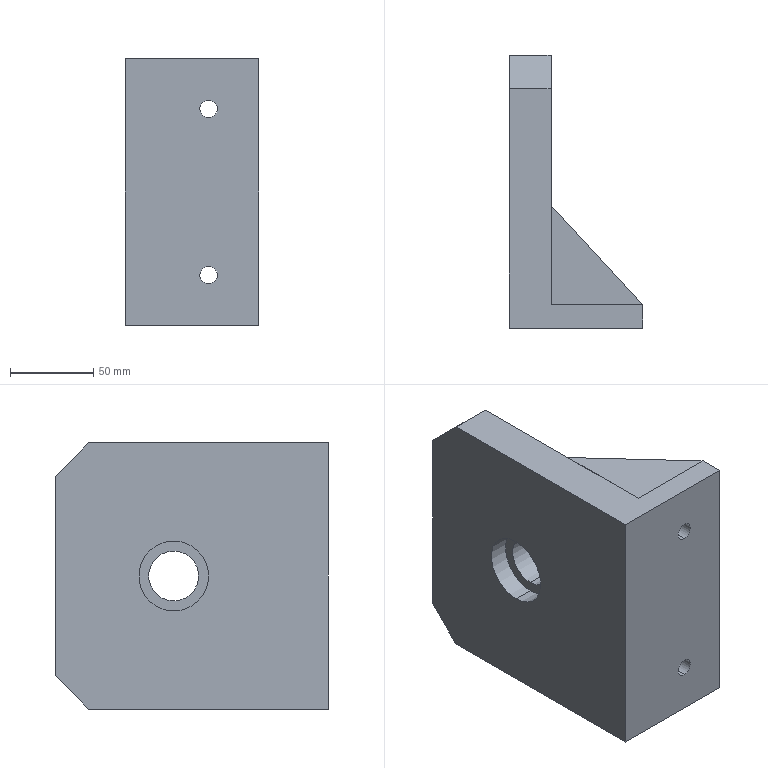Part | SolidWorks | features ICE 5, Chamfer 1, Extrusion 1, HoleWzd 1 | 3 solids | 29 faces | box 80 x 164 x 160 mm | volume 773961 mm3 | plane 21 | cylinder 8 | commonest cylinder face diameters 10.5 x4 30 x2 42 x2
STEP:
#1=CARTESIAN_POINT('',(-15.,74.,80.));
#2=VERTEX_POINT('',#1);
#3=CARTESIAN_POINT('',(-15.,14.,80.));
#4=VERTEX_POINT('',#3);
#5=CARTESIAN_POINT('',(-15.,74.,80.));
#6=DIRECTION('',(0.,-1.,0.));
#7=VECTOR('',#6,1000.);
#8=LINE('',#5,#7);
#9=EDGE_CURVE('',#2,#4,#8,.T.);
#10=ORIENTED_EDGE('',*,*,#9,.F.);
#11=CARTESIAN_POINT('',(-15.,74.,70.));
#12=VERTEX_POINT('',#11);
#13=CARTESIAN_POINT('',(-15.,74.,70.));
#14=DIRECTION('',(0.,0.,1.));
#15=VECTOR('',#14,1000.);
#16=LINE('',#13,#15);
#17=EDGE_CURVE('',#12,#2,#16,.T.);
#18=ORIENTED_EDGE('',*,*,#17,.F.);
#19=CARTESIAN_POINT('',(-15.,14.,70.));
#20=VERTEX_POINT('',#19);
#21=CARTESIAN_POINT('',(-15.,74.,70.));
#22=DIRECTION('',(0.,-1.,0.));
#23=VECTOR('',#22,1000.);
#24=LINE('',#21,#23);
#25=EDGE_CURVE('',#12,#20,#24,.T.);
#26=ORIENTED_EDGE('',*,*,#25,.T.);
#27=CARTESIAN_POINT('',(-15.,14.,70.));
#28=DIRECTION('',(0.,0.,1.));
#29=VECTOR('',#28,1000.);
#30=LINE('',#27,#29);
#31=EDGE_CURVE('',#20,#4,#30,.T.);
#32=ORIENTED_EDGE('',*,*,#31,.T.);
#33=EDGE_LOOP('',(#10,#18,#26,#32));
#34=FACE_OUTER_BOUND('',#33,.T.);
#35=CARTESIAN_POINT('',(-15.,74.,70.));
#36=DIRECTION('',(-1.,0.,0.));
#37=DIRECTION('',(0.,-1.,0.));
#38=AXIS2_PLACEMENT_3D('',#35,#36,#37);
#39=PLANE('',#38);
#40=ADVANCED_FACE('',(#34),#39,.T.);
#41=CARTESIAN_POINT('',(40.,14.,80.));
#42=VERTEX_POINT('',#41);
#43=CARTESIAN_POINT('',(-15.,74.,80.));
#44=DIRECTION('',(-0.6757,0.7372,0.));
#45=VECTOR('',#44,1000.);
#46=LINE('',#43,#45);
#47=EDGE_CURVE('',#42,#2,#46,.T.);
#48=ORIENTED_EDGE('',*,*,#47,.F.);
#49=CARTESIAN_POINT('',(40.,14.,70.));
#50=VERTEX_POINT('',#49);
#51=CARTESIAN_POINT('',(40.,14.,70.));
#52=DIRECTION('',(0.,0.,1.));
#53=VECTOR('',#52,1000.);
#54=LINE('',#51,#53);
#55=EDGE_CURVE('',#50,#42,#54,.T.);
#56=ORIENTED_EDGE('',*,*,#55,.F.);
#57=CARTESIAN_POINT('',(-15.,74.,70.));
#58=DIRECTION('',(-0.6757,0.7372,0.));
#59=VECTOR('',#58,1000.);
#60=LINE('',#57,#59);
#61=EDGE_CURVE('',#50,#12,#60,.T.);
#62=ORIENTED_EDGE('',*,*,#61,.T.);
#63=ORIENTED_EDGE('',*,*,#17,.T.);
#64=EDGE_LOOP('',(#48,#56,#62,#63));
#65=FACE_OUTER_BOUND('',#64,.T.);
#66=CARTESIAN_POINT('',(-15.,74.,70.));
#67=DIRECTION('',(0.7372,0.6757,0.));
#68=DIRECTION('',(-0.6757,0.7372,0.));
#69=AXIS2_PLACEMENT_3D('',#66,#67,#68);
#70=PLANE('',#69);
#71=ADVANCED_FACE('',(#65),#70,.T.);
#72=CARTESIAN_POINT('',(-15.,14.,80.));
#73=DIRECTION('',(1.,0.,0.));
#74=VECTOR('',#73,1000.);
#75=LINE('',#72,#74);
#76=EDGE_CURVE('',#4,#42,#75,.T.);
#77=ORIENTED_EDGE('',*,*,#76,.F.);
#78=ORIENTED_EDGE('',*,*,#31,.F.);
#79=CARTESIAN_POINT('',(-15.,14.,70.));
#80=DIRECTION('',(1.,0.,0.));
#81=VECTOR('',#80,1000.);
#82=LINE('',#79,#81);
#83=EDGE_CURVE('',#20,#50,#82,.T.);
#84=ORIENTED_EDGE('',*,*,#83,.T.);
#85=ORIENTED_EDGE('',*,*,#55,.T.);
#86=EDGE_LOOP('',(#77,#78,#84,#85));
#87=FACE_OUTER_BOUND('',#86,.T.);
#88=CARTESIAN_POINT('',(-15.,14.,70.));
#89=DIRECTION('',(0.,-1.,0.));
#90=DIRECTION('',(0.,0.,-1.));
#91=AXIS2_PLACEMENT_3D('',#88,#89,#90);
#92=PLANE('',#91);
#93=ADVANCED_FACE('',(#87),#92,.T.);
#94=ORIENTED_EDGE('',*,*,#25,.F.);
#95=ORIENTED_EDGE('',*,*,#61,.F.);
#96=ORIENTED_EDGE('',*,*,#83,.F.);
#97=EDGE_LOOP('',(#94,#95,#96));
#98=FACE_OUTER_BOUND('',#97,.T.);
#99=CARTESIAN_POINT('',(0.,0.,70.));
#100=DIRECTION('',(0.,0.,1.));
#101=DIRECTION('',(1.,0.,0.));
#102=AXIS2_PLACEMENT_3D('',#99,#100,#101);
#103=PLANE('',#102);
#104=ADVANCED_FACE('',(#98),#103,.F.);
#105=ORIENTED_EDGE('',*,*,#9,.T.);
#106=ORIENTED_EDGE('',*,*,#76,.T.);
#107=ORIENTED_EDGE('',*,*,#47,.T.);
#108=EDGE_LOOP('',(#105,#106,#107));
#109=FACE_OUTER_BOUND('',#108,.T.);
#110=CARTESIAN_POINT('',(0.,0.,80.));
#111=DIRECTION('',(0.,0.,1.));
#112=DIRECTION('',(1.,0.,0.));
#113=AXIS2_PLACEMENT_3D('',#110,#111,#112);
#114=PLANE('',#113);
#115=ADVANCED_FACE('',(#109),#114,.T.);
#116=CLOSED_SHELL('',(#40,#71,#93,#104,#115));
#117=MANIFOLD_SOLID_BREP('',#116);
#118=CARTESIAN_POINT('',(-15.,74.,-80.));
#119=VERTEX_POINT('',#118);
#120=CARTESIAN_POINT('',(40.,14.,-80.));
#121=VERTEX_POINT('',#120);
#122=CARTESIAN_POINT('',(-15.,74.,-80.));
#123=DIRECTION('',(0.6757,-0.7372,0.));
#124=VECTOR('',#123,1000.);
#125=LINE('',#122,#124);
#126=EDGE_CURVE('',#119,#121,#125,.T.);
#127=ORIENTED_EDGE('',*,*,#126,.F.);
#128=CARTESIAN_POINT('',(-15.,74.,-70.));
#129=VERTEX_POINT('',#128);
#130=CARTESIAN_POINT('',(-15.,74.,-70.));
#131=DIRECTION('',(0.,0.,-1.));
#132=VECTOR('',#131,1000.);
#133=LINE('',#130,#132);
#134=EDGE_CURVE('',#129,#119,#133,.T.);
#135=ORIENTED_EDGE('',*,*,#134,.F.);
#136=CARTESIAN_POINT('',(40.,14.,-70.));
#137=VERTEX_POINT('',#136);
#138=CARTESIAN_POINT('',(-15.,74.,-70.));
#139=DIRECTION('',(0.6757,-0.7372,0.));
#140=VECTOR('',#139,1000.);
#141=LINE('',#138,#140);
#142=EDGE_CURVE('',#129,#137,#141,.T.);
#143=ORIENTED_EDGE('',*,*,#142,.T.);
#144=CARTESIAN_POINT('',(40.,14.,-70.));
#145=DIRECTION('',(0.,0.,-1.));
#146=VECTOR('',#145,1000.);
#147=LINE('',#144,#146);
#148=EDGE_CURVE('',#137,#121,#147,.T.);
#149=ORIENTED_EDGE('',*,*,#148,.T.);
#150=EDGE_LOOP('',(#127,#135,#143,#149));
#151=FACE_OUTER_BOUND('',#150,.T.);
#152=CARTESIAN_POINT('',(-15.,74.,-70.));
#153=DIRECTION('',(0.7372,0.6757,0.));
#154=DIRECTION('',(-0.6757,0.7372,0.));
#155=AXIS2_PLACEMENT_3D('',#152,#153,#154);
#156=PLANE('',#155);
#157=ADVANCED_FACE('',(#151),#156,.T.);
#158=CARTESIAN_POINT('',(-15.,14.,-80.));
#159=VERTEX_POINT('',#158);
#160=CARTESIAN_POINT('',(-15.,14.,-80.));
#161=DIRECTION('',(0.,1.,0.));
#162=VECTOR('',#161,1000.);
#163=LINE('',#160,#162);
#164=EDGE_CURVE('',#159,#119,#163,.T.);
#165=ORIENTED_EDGE('',*,*,#164,.F.);
#166=CARTESIAN_POINT('',(-15.,14.,-70.));
#167=VERTEX_POINT('',#166);
#168=CARTESIAN_POINT('',(-15.,14.,-70.));
#169=DIRECTION('',(0.,0.,-1.));
#170=VECTOR('',#169,1000.);
#171=LINE('',#168,#170);
#172=EDGE_CURVE('',#167,#159,#171,.T.);
#173=ORIENTED_EDGE('',*,*,#172,.F.);
#174=CARTESIAN_POINT('',(-15.,14.,-70.));
#175=DIRECTION('',(0.,1.,0.));
#176=VECTOR('',#175,1000.);
#177=LINE('',#174,#176);
#178=EDGE_CURVE('',#167,#129,#177,.T.);
#179=ORIENTED_EDGE('',*,*,#178,.T.);
#180=ORIENTED_EDGE('',*,*,#134,.T.);
#181=EDGE_LOOP('',(#165,#173,#179,#180));
#182=FACE_OUTER_BOUND('',#181,.T.);
#183=CARTESIAN_POINT('',(-15.,14.,-70.));
#184=DIRECTION('',(-1.,0.,0.));
#185=DIRECTION('',(0.,-1.,0.));
#186=AXIS2_PLACEMENT_3D('',#183,#184,#185);
#187=PLANE('',#186);
#188=ADVANCED_FACE('',(#182),#187,.T.);
#189=CARTESIAN_POINT('',(40.,14.,-80.));
#190=DIRECTION('',(-1.,0.,0.));
#191=VECTOR('',#190,1000.);
#192=LINE('',#189,#191);
#193=EDGE_CURVE('',#121,#159,#192,.T.);
#194=ORIENTED_EDGE('',*,*,#193,.F.);
#195=ORIENTED_EDGE('',*,*,#148,.F.);
#196=CARTESIAN_POINT('',(40.,14.,-70.));
#197=DIRECTION('',(-1.,0.,0.));
#198=VECTOR('',#197,1000.);
#199=LINE('',#196,#198);
#200=EDGE_CURVE('',#137,#167,#199,.T.);
#201=ORIENTED_EDGE('',*,*,#200,.T.);
#202=ORIENTED_EDGE('',*,*,#172,.T.);
#203=EDGE_LOOP('',(#194,#195,#201,#202));
#204=FACE_OUTER_BOUND('',#203,.T.);
#205=CARTESIAN_POINT('',(40.,14.,-70.));
#206=DIRECTION('',(0.,-1.,0.));
#207=DIRECTION('',(0.,0.,-1.));
#208=AXIS2_PLACEMENT_3D('',#205,#206,#207);
#209=PLANE('',#208);
#210=ADVANCED_FACE('',(#204),#209,.T.);
#211=ORIENTED_EDGE('',*,*,#142,.F.);
#212=ORIENTED_EDGE('',*,*,#178,.F.);
#213=ORIENTED_EDGE('',*,*,#200,.F.);
#214=EDGE_LOOP('',(#211,#212,#213));
#215=FACE_OUTER_BOUND('',#214,.T.);
#216=CARTESIAN_POINT('',(0.,0.,-70.));
#217=DIRECTION('',(0.,0.,-1.));
#218=DIRECTION('',(-1.,0.,0.));
#219=AXIS2_PLACEMENT_3D('',#216,#217,#218);
#220=PLANE('',#219);
#221=ADVANCED_FACE('',(#215),#220,.F.);
#222=ORIENTED_EDGE('',*,*,#126,.T.);
#223=ORIENTED_EDGE('',*,*,#193,.T.);
#224=ORIENTED_EDGE('',*,*,#164,.T.);
#225=EDGE_LOOP('',(#222,#223,#224));
#226=FACE_OUTER_BOUND('',#225,.T.);
#227=CARTESIAN_POINT('',(0.,0.,-80.));
#228=DIRECTION('',(0.,0.,-1.));
#229=DIRECTION('',(-1.,0.,0.));
#230=AXIS2_PLACEMENT_3D('',#227,#228,#229);
#231=PLANE('',#230);
#232=ADVANCED_FACE('',(#226),#231,.T.);
#233=CLOSED_SHELL('',(#157,#188,#210,#221,#232));
#234=MANIFOLD_SOLID_BREP('',#233);
#235=CARTESIAN_POINT('',(10.,0.,-55.25));
#236=VERTEX_POINT('',#235);
#237=CARTESIAN_POINT('',(10.,0.,-44.75));
#238=VERTEX_POINT('',#237);
#239=CARTESIAN_POINT('',(10.,0.,-50.));
#240=DIRECTION('',(0.,1.,0.));
#241=DIRECTION('',(0.,0.,1.));
#242=AXIS2_PLACEMENT_3D('',#239,#240,#241);
#243=CIRCLE('',#242,5.25);
#244=EDGE_CURVE('',#236,#238,#243,.T.);
#245=ORIENTED_EDGE('',*,*,#244,.F.);
#246=CARTESIAN_POINT('',(10.,14.,-55.25));
#247=VERTEX_POINT('',#246);
#248=CARTESIAN_POINT('',(10.,14.,-55.25));
#249=DIRECTION('',(0.,1.,0.));
#250=VECTOR('',#249,1000.);
#251=LINE('',#248,#250);
#252=EDGE_CURVE('',#236,#247,#251,.T.);
#253=ORIENTED_EDGE('',*,*,#252,.T.);
#254=CARTESIAN_POINT('',(10.,14.,-44.75));
#255=VERTEX_POINT('',#254);
#256=CARTESIAN_POINT('',(10.,14.,-50.));
#257=DIRECTION('',(0.,1.,0.));
#258=DIRECTION('',(0.,0.,1.));
#259=AXIS2_PLACEMENT_3D('',#256,#257,#258);
#260=CIRCLE('',#259,5.25);
#261=EDGE_CURVE('',#247,#255,#260,.T.);
#262=ORIENTED_EDGE('',*,*,#261,.T.);
#263=CARTESIAN_POINT('',(10.,14.,-44.75));
#264=DIRECTION('',(0.,1.,0.));
#265=VECTOR('',#264,1000.);
#266=LINE('',#263,#265);
#267=EDGE_CURVE('',#238,#255,#266,.T.);
#268=ORIENTED_EDGE('',*,*,#267,.F.);
#269=EDGE_LOOP('',(#245,#253,#262,#268));
#270=FACE_OUTER_BOUND('',#269,.T.);
#271=CARTESIAN_POINT('',(10.,14.,-50.));
#272=DIRECTION('',(0.,1.,0.));
#273=DIRECTION('',(0.,0.,1.));
#274=AXIS2_PLACEMENT_3D('',#271,#272,#273);
#275=CYLINDRICAL_SURFACE('',#274,5.25);
#276=ADVANCED_FACE('',(#270),#275,.F.);
#277=CARTESIAN_POINT('',(10.,0.,44.75));
#278=VERTEX_POINT('',#277);
#279=CARTESIAN_POINT('',(10.,0.,55.25));
#280=VERTEX_POINT('',#279);
#281=CARTESIAN_POINT('',(10.,0.,50.));
#282=DIRECTION('',(0.,1.,0.));
#283=DIRECTION('',(0.,0.,1.));
#284=AXIS2_PLACEMENT_3D('',#281,#282,#283);
#285=CIRCLE('',#284,5.25);
#286=EDGE_CURVE('',#278,#280,#285,.T.);
#287=ORIENTED_EDGE('',*,*,#286,.F.);
#288=CARTESIAN_POINT('',(10.,14.,44.75));
#289=VERTEX_POINT('',#288);
#290=CARTESIAN_POINT('',(10.,14.,44.75));
#291=DIRECTION('',(0.,1.,0.));
#292=VECTOR('',#291,1000.);
#293=LINE('',#290,#292);
#294=EDGE_CURVE('',#278,#289,#293,.T.);
#295=ORIENTED_EDGE('',*,*,#294,.T.);
#296=CARTESIAN_POINT('',(10.,14.,55.25));
#297=VERTEX_POINT('',#296);
#298=CARTESIAN_POINT('',(10.,14.,50.));
#299=DIRECTION('',(0.,1.,0.));
#300=DIRECTION('',(0.,0.,1.));
#301=AXIS2_PLACEMENT_3D('',#298,#299,#300);
#302=CIRCLE('',#301,5.25);
#303=EDGE_CURVE('',#289,#297,#302,.T.);
#304=ORIENTED_EDGE('',*,*,#303,.T.);
#305=CARTESIAN_POINT('',(10.,14.,55.25));
#306=DIRECTION('',(0.,1.,0.));
#307=VECTOR('',#306,1000.);
#308=LINE('',#305,#307);
#309=EDGE_CURVE('',#280,#297,#308,.T.);
#310=ORIENTED_EDGE('',*,*,#309,.F.);
#311=EDGE_LOOP('',(#287,#295,#304,#310));
#312=FACE_OUTER_BOUND('',#311,.T.);
#313=CARTESIAN_POINT('',(10.,14.,50.));
#314=DIRECTION('',(0.,1.,0.));
#315=DIRECTION('',(0.,0.,1.));
#316=AXIS2_PLACEMENT_3D('',#313,#314,#315);
#317=CYLINDRICAL_SURFACE('',#316,5.25);
#318=ADVANCED_FACE('',(#312),#317,.F.);
#319=CARTESIAN_POINT('',(-15.,93.,-15.));
#320=VERTEX_POINT('',#319);
#321=CARTESIAN_POINT('',(-15.,93.,15.));
#322=VERTEX_POINT('',#321);
#323=CARTESIAN_POINT('',(-15.,93.,0.));
#324=DIRECTION('',(-1.,0.,0.));
#325=DIRECTION('',(0.,0.,1.));
#326=AXIS2_PLACEMENT_3D('',#323,#324,#325);
#327=CIRCLE('',#326,15.);
#328=EDGE_CURVE('',#320,#322,#327,.T.);
#329=ORIENTED_EDGE('',*,*,#328,.F.);
#330=CARTESIAN_POINT('',(-28.,93.,-15.));
#331=VERTEX_POINT('',#330);
#332=CARTESIAN_POINT('',(40.,93.,-15.));
#333=DIRECTION('',(-1.,0.,0.));
#334=VECTOR('',#333,1000.);
#335=LINE('',#332,#334);
#336=EDGE_CURVE('',#320,#331,#335,.T.);
#337=ORIENTED_EDGE('',*,*,#336,.T.);
#338=CARTESIAN_POINT('',(-28.,93.,15.));
#339=VERTEX_POINT('',#338);
#340=CARTESIAN_POINT('',(-28.,93.,0.));
#341=DIRECTION('',(-1.,0.,0.));
#342=DIRECTION('',(0.,0.,1.));
#343=AXIS2_PLACEMENT_3D('',#340,#341,#342);
#344=CIRCLE('',#343,15.);
#345=EDGE_CURVE('',#331,#339,#344,.T.);
#346=ORIENTED_EDGE('',*,*,#345,.T.);
#347=CARTESIAN_POINT('',(40.,93.,15.));
#348=DIRECTION('',(-1.,0.,0.));
#349=VECTOR('',#348,1000.);
#350=LINE('',#347,#349);
#351=EDGE_CURVE('',#322,#339,#350,.T.);
#352=ORIENTED_EDGE('',*,*,#351,.F.);
#353=EDGE_LOOP('',(#329,#337,#346,#352));
#354=FACE_OUTER_BOUND('',#353,.T.);
#355=CARTESIAN_POINT('',(40.,93.,0.));
#356=DIRECTION('',(-1.,0.,0.));
#357=DIRECTION('',(0.,0.,1.));
#358=AXIS2_PLACEMENT_3D('',#355,#356,#357);
#359=CYLINDRICAL_SURFACE('',#358,15.);
#360=ADVANCED_FACE('',(#354),#359,.F.);
#361=CARTESIAN_POINT('',(-28.,93.,-21.));
#362=VERTEX_POINT('',#361);
#363=CARTESIAN_POINT('',(-28.,93.,21.));
#364=VERTEX_POINT('',#363);
#365=CARTESIAN_POINT('',(-28.,93.,0.));
#366=DIRECTION('',(-1.,0.,0.));
#367=DIRECTION('',(0.,0.,1.));
#368=AXIS2_PLACEMENT_3D('',#365,#366,#367);
#369=CIRCLE('',#368,21.);
#370=EDGE_CURVE('',#362,#364,#369,.T.);
#371=ORIENTED_EDGE('',*,*,#370,.F.);
#372=CARTESIAN_POINT('',(-40.,93.,-21.));
#373=VERTEX_POINT('',#372);
#374=CARTESIAN_POINT('',(-28.,93.,-21.));
#375=DIRECTION('',(-1.,0.,0.));
#376=VECTOR('',#375,1000.);
#377=LINE('',#374,#376);
#378=EDGE_CURVE('',#362,#373,#377,.T.);
#379=ORIENTED_EDGE('',*,*,#378,.T.);
#380=CARTESIAN_POINT('',(-40.,93.,21.));
#381=VERTEX_POINT('',#380);
#382=CARTESIAN_POINT('',(-40.,93.,0.));
#383=DIRECTION('',(-1.,0.,0.));
#384=DIRECTION('',(0.,0.,1.));
#385=AXIS2_PLACEMENT_3D('',#382,#383,#384);
#386=CIRCLE('',#385,21.);
#387=EDGE_CURVE('',#373,#381,#386,.T.);
#388=ORIENTED_EDGE('',*,*,#387,.T.);
#389=CARTESIAN_POINT('',(-28.,93.,21.));
#390=DIRECTION('',(-1.,0.,0.));
#391=VECTOR('',#390,1000.);
#392=LINE('',#389,#391);
#393=EDGE_CURVE('',#364,#381,#392,.T.);
#394=ORIENTED_EDGE('',*,*,#393,.F.);
#395=EDGE_LOOP('',(#371,#379,#388,#394));
#396=FACE_OUTER_BOUND('',#395,.T.);
#397=CARTESIAN_POINT('',(-28.,93.,0.));
#398=DIRECTION('',(-1.,0.,0.));
#399=DIRECTION('',(0.,0.,1.));
#400=AXIS2_PLACEMENT_3D('',#397,#398,#399);
#401=CYLINDRICAL_SURFACE('',#400,21.);
#402=ADVANCED_FACE('',(#396),#401,.F.);
#403=CARTESIAN_POINT('',(40.,0.,80.));
#404=VERTEX_POINT('',#403);
#405=CARTESIAN_POINT('',(40.,0.,-80.));
#406=VERTEX_POINT('',#405);
#407=CARTESIAN_POINT('',(40.,0.,-80.));
#408=DIRECTION('',(0.,0.,-1.));
#409=VECTOR('',#408,1000.);
#410=LINE('',#407,#409);
#411=EDGE_CURVE('',#404,#406,#410,.T.);
#412=ORIENTED_EDGE('',*,*,#411,.T.);
#413=CARTESIAN_POINT('',(40.,14.,-80.));
#414=VERTEX_POINT('',#413);
#415=CARTESIAN_POINT('',(40.,14.,-80.));
#416=DIRECTION('',(0.,-1.,0.));
#417=VECTOR('',#416,1000.);
#418=LINE('',#415,#417);
#419=EDGE_CURVE('',#414,#406,#418,.T.);
#420=ORIENTED_EDGE('',*,*,#419,.F.);
#421=CARTESIAN_POINT('',(40.,14.,80.));
#422=VERTEX_POINT('',#421);
#423=CARTESIAN_POINT('',(40.,14.,-80.));
#424=DIRECTION('',(0.,0.,-1.));
#425=VECTOR('',#424,1000.);
#426=LINE('',#423,#425);
#427=EDGE_CURVE('',#422,#414,#426,.T.);
#428=ORIENTED_EDGE('',*,*,#427,.F.);
#429=CARTESIAN_POINT('',(40.,14.,80.));
#430=DIRECTION('',(0.,-1.,0.));
#431=VECTOR('',#430,1000.);
#432=LINE('',#429,#431);
#433=EDGE_CURVE('',#422,#404,#432,.T.);
#434=ORIENTED_EDGE('',*,*,#433,.T.);
#435=EDGE_LOOP('',(#412,#420,#428,#434));
#436=FACE_OUTER_BOUND('',#435,.T.);
#437=CARTESIAN_POINT('',(40.,14.,-80.));
#438=DIRECTION('',(-1.,0.,0.));
#439=DIRECTION('',(0.,0.,1.));
#440=AXIS2_PLACEMENT_3D('',#437,#438,#439);
#441=PLANE('',#440);
#442=ADVANCED_FACE('',(#436),#441,.F.);
#443=CARTESIAN_POINT('',(-40.,144.,-80.));
#444=VERTEX_POINT('',#443);
#445=CARTESIAN_POINT('',(-40.,0.,-80.));
#446=VERTEX_POINT('',#445);
#447=CARTESIAN_POINT('',(-40.,14.,-80.));
#448=DIRECTION('',(0.,-1.,0.));
#449=VECTOR('',#448,1000.);
#450=LINE('',#447,#449);
#451=EDGE_CURVE('',#444,#446,#450,.T.);
#452=ORIENTED_EDGE('',*,*,#451,.F.);
#453=CARTESIAN_POINT('',(-15.,144.,-80.));
#454=VERTEX_POINT('',#453);
#455=CARTESIAN_POINT('',(-15.,144.,-80.));
#456=DIRECTION('',(1.,0.,0.));
#457=VECTOR('',#456,1000.);
#458=LINE('',#455,#457);
#459=EDGE_CURVE('',#444,#454,#458,.T.);
#460=ORIENTED_EDGE('',*,*,#459,.T.);
#461=CARTESIAN_POINT('',(-15.,14.,-80.));
#462=VERTEX_POINT('',#461);
#463=CARTESIAN_POINT('',(-15.,164.,-80.));
#464=DIRECTION('',(0.,-1.,0.));
#465=VECTOR('',#464,1000.);
#466=LINE('',#463,#465);
#467=EDGE_CURVE('',#454,#462,#466,.T.);
#468=ORIENTED_EDGE('',*,*,#467,.T.);
#469=CARTESIAN_POINT('',(-40.,14.,-80.));
#470=DIRECTION('',(-1.,0.,0.));
#471=VECTOR('',#470,1000.);
#472=LINE('',#469,#471);
#473=EDGE_CURVE('',#414,#462,#472,.T.);
#474=ORIENTED_EDGE('',*,*,#473,.F.);
#475=ORIENTED_EDGE('',*,*,#419,.T.);
#476=CARTESIAN_POINT('',(-40.,0.,-80.));
#477=DIRECTION('',(-1.,0.,0.));
#478=VECTOR('',#477,1000.);
#479=LINE('',#476,#478);
#480=EDGE_CURVE('',#406,#446,#479,.T.);
#481=ORIENTED_EDGE('',*,*,#480,.T.);
#482=EDGE_LOOP('',(#452,#460,#468,#474,#475,#481));
#483=FACE_OUTER_BOUND('',#482,.T.);
#484=CARTESIAN_POINT('',(-40.,14.,-80.));
#485=DIRECTION('',(0.,0.,1.));
#486=DIRECTION('',(1.,0.,0.));
#487=AXIS2_PLACEMENT_3D('',#484,#485,#486);
#488=PLANE('',#487);
#489=ADVANCED_FACE('',(#483),#488,.F.);
#490=CARTESIAN_POINT('',(-40.,93.,0.));
#491=DIRECTION('',(-1.,0.,0.));
#492=DIRECTION('',(0.,0.,1.));
#493=AXIS2_PLACEMENT_3D('',#490,#491,#492);
#494=CIRCLE('',#493,21.);
#495=EDGE_CURVE('',#381,#373,#494,.T.);
#496=ORIENTED_EDGE('',*,*,#495,.F.);
#497=ORIENTED_EDGE('',*,*,#387,.F.);
#498=EDGE_LOOP('',(#496,#497));
#499=FACE_BOUND('',#498,.T.);
#500=CARTESIAN_POINT('',(-40.,144.,80.));
#501=VERTEX_POINT('',#500);
#502=CARTESIAN_POINT('',(-40.,0.,80.));
#503=VERTEX_POINT('',#502);
#504=CARTESIAN_POINT('',(-40.,14.,80.));
#505=DIRECTION('',(0.,-1.,0.));
#506=VECTOR('',#505,1000.);
#507=LINE('',#504,#506);
#508=EDGE_CURVE('',#501,#503,#507,.T.);
#509=ORIENTED_EDGE('',*,*,#508,.F.);
#510=CARTESIAN_POINT('',(-40.,164.,60.));
#511=VERTEX_POINT('',#510);
#512=CARTESIAN_POINT('',(-40.,164.,60.));
#513=DIRECTION('',(0.,0.7071,-0.7071));
#514=VECTOR('',#513,1000.);
#515=LINE('',#512,#514);
#516=EDGE_CURVE('',#501,#511,#515,.T.);
#517=ORIENTED_EDGE('',*,*,#516,.T.);
#518=CARTESIAN_POINT('',(-40.,164.,-60.));
#519=VERTEX_POINT('',#518);
#520=CARTESIAN_POINT('',(-40.,164.,-80.));
#521=DIRECTION('',(0.,0.,1.));
#522=VECTOR('',#521,1000.);
#523=LINE('',#520,#522);
#524=EDGE_CURVE('',#519,#511,#523,.T.);
#525=ORIENTED_EDGE('',*,*,#524,.F.);
#526=CARTESIAN_POINT('',(-40.,164.,-60.));
#527=DIRECTION('',(0.,-0.7071,-0.7071));
#528=VECTOR('',#527,1000.);
#529=LINE('',#526,#528);
#530=EDGE_CURVE('',#519,#444,#529,.T.);
#531=ORIENTED_EDGE('',*,*,#530,.T.);
#532=ORIENTED_EDGE('',*,*,#451,.T.);
#533=CARTESIAN_POINT('',(-40.,0.,-80.));
#534=DIRECTION('',(0.,0.,1.));
#535=VECTOR('',#534,1000.);
#536=LINE('',#533,#535);
#537=EDGE_CURVE('',#446,#503,#536,.T.);
#538=ORIENTED_EDGE('',*,*,#537,.T.);
#539=EDGE_LOOP('',(#509,#517,#525,#531,#532,#538));
#540=FACE_OUTER_BOUND('',#539,.T.);
#541=CARTESIAN_POINT('',(-40.,14.,-80.));
#542=DIRECTION('',(1.,0.,0.));
#543=DIRECTION('',(0.,0.,-1.));
#544=AXIS2_PLACEMENT_3D('',#541,#542,#543);
#545=PLANE('',#544);
#546=ADVANCED_FACE('',(#499,#540),#545,.F.);
#547=CARTESIAN_POINT('',(-15.,144.,80.));
#548=VERTEX_POINT('',#547);
#549=CARTESIAN_POINT('',(-15.,14.,80.));
#550=VERTEX_POINT('',#549);
#551=CARTESIAN_POINT('',(-15.,164.,80.));
#552=DIRECTION('',(0.,-1.,0.));
#553=VECTOR('',#552,1000.);
#554=LINE('',#551,#553);
#555=EDGE_CURVE('',#548,#550,#554,.T.);
#556=ORIENTED_EDGE('',*,*,#555,.F.);
#557=CARTESIAN_POINT('',(-40.,144.,80.));
#558=DIRECTION('',(-1.,0.,0.));
#559=VECTOR('',#558,1000.);
#560=LINE('',#557,#559);
#561=EDGE_CURVE('',#548,#501,#560,.T.);
#562=ORIENTED_EDGE('',*,*,#561,.T.);
#563=ORIENTED_EDGE('',*,*,#508,.T.);
#564=CARTESIAN_POINT('',(-40.,0.,80.));
#565=DIRECTION('',(1.,0.,0.));
#566=VECTOR('',#565,1000.);
#567=LINE('',#564,#566);
#568=EDGE_CURVE('',#503,#404,#567,.T.);
#569=ORIENTED_EDGE('',*,*,#568,.T.);
#570=ORIENTED_EDGE('',*,*,#433,.F.);
#571=CARTESIAN_POINT('',(-40.,14.,80.));
#572=DIRECTION('',(1.,0.,0.));
#573=VECTOR('',#572,1000.);
#574=LINE('',#571,#573);
#575=EDGE_CURVE('',#550,#422,#574,.T.);
#576=ORIENTED_EDGE('',*,*,#575,.F.);
#577=EDGE_LOOP('',(#556,#562,#563,#569,#570,#576));
#578=FACE_OUTER_BOUND('',#577,.T.);
#579=CARTESIAN_POINT('',(-40.,14.,80.));
#580=DIRECTION('',(0.,0.,-1.));
#581=DIRECTION('',(-1.,0.,0.));
#582=AXIS2_PLACEMENT_3D('',#579,#580,#581);
#583=PLANE('',#582);
#584=ADVANCED_FACE('',(#578),#583,.F.);
#585=CARTESIAN_POINT('',(10.,14.,-50.));
#586=DIRECTION('',(0.,1.,0.));
#587=DIRECTION('',(0.,0.,1.));
#588=AXIS2_PLACEMENT_3D('',#585,#586,#587);
#589=CIRCLE('',#588,5.25);
#590=EDGE_CURVE('',#255,#247,#589,.T.);
#591=ORIENTED_EDGE('',*,*,#590,.F.);
#592=ORIENTED_EDGE('',*,*,#261,.F.);
#593=EDGE_LOOP('',(#591,#592));
#594=FACE_BOUND('',#593,.T.);
#595=CARTESIAN_POINT('',(10.,14.,50.));
#596=DIRECTION('',(0.,1.,0.));
#597=DIRECTION('',(0.,0.,1.));
#598=AXIS2_PLACEMENT_3D('',#595,#596,#597);
#599=CIRCLE('',#598,5.25);
#600=EDGE_CURVE('',#297,#289,#599,.T.);
#601=ORIENTED_EDGE('',*,*,#600,.F.);
#602=ORIENTED_EDGE('',*,*,#303,.F.);
#603=EDGE_LOOP('',(#601,#602));
#604=FACE_BOUND('',#603,.T.);
#605=CARTESIAN_POINT('',(-15.,14.,-80.));
#606=DIRECTION('',(0.,0.,-1.));
#607=VECTOR('',#606,1000.);
#608=LINE('',#605,#607);
#609=EDGE_CURVE('',#550,#462,#608,.T.);
#610=ORIENTED_EDGE('',*,*,#609,.F.);
#611=ORIENTED_EDGE('',*,*,#575,.T.);
#612=ORIENTED_EDGE('',*,*,#427,.T.);
#613=ORIENTED_EDGE('',*,*,#473,.T.);
#614=EDGE_LOOP('',(#610,#611,#612,#613));
#615=FACE_OUTER_BOUND('',#614,.T.);
#616=CARTESIAN_POINT('',(0.,14.,0.));
#617=DIRECTION('',(0.,1.,0.));
#618=DIRECTION('',(0.,0.,1.));
#619=AXIS2_PLACEMENT_3D('',#616,#617,#618);
#620=PLANE('',#619);
#621=ADVANCED_FACE('',(#594,#604,#615),#620,.T.);
#622=CARTESIAN_POINT('',(10.,0.,-50.));
#623=DIRECTION('',(0.,1.,0.));
#624=DIRECTION('',(0.,0.,1.));
#625=AXIS2_PLACEMENT_3D('',#622,#623,#624);
#626=CIRCLE('',#625,5.25);
#627=EDGE_CURVE('',#238,#236,#626,.T.);
#628=ORIENTED_EDGE('',*,*,#627,.T.);
#629=ORIENTED_EDGE('',*,*,#244,.T.);
#630=EDGE_LOOP('',(#628,#629));
#631=FACE_BOUND('',#630,.T.);
#632=CARTESIAN_POINT('',(10.,0.,50.));
#633=DIRECTION('',(0.,1.,0.));
#634=DIRECTION('',(0.,0.,1.));
#635=AXIS2_PLACEMENT_3D('',#632,#633,#634);
#636=CIRCLE('',#635,5.25);
#637=EDGE_CURVE('',#280,#278,#636,.T.);
#638=ORIENTED_EDGE('',*,*,#637,.T.);
#639=ORIENTED_EDGE('',*,*,#286,.T.);
#640=EDGE_LOOP('',(#638,#639));
#641=FACE_BOUND('',#640,.T.);
#642=ORIENTED_EDGE('',*,*,#411,.F.);
#643=ORIENTED_EDGE('',*,*,#568,.F.);
#644=ORIENTED_EDGE('',*,*,#537,.F.);
#645=ORIENTED_EDGE('',*,*,#480,.F.);
#646=EDGE_LOOP('',(#642,#643,#644,#645));
#647=FACE_OUTER_BOUND('',#646,.T.);
#648=CARTESIAN_POINT('',(0.,0.,0.));
#649=DIRECTION('',(0.,1.,0.));
#650=DIRECTION('',(0.,0.,1.));
#651=AXIS2_PLACEMENT_3D('',#648,#649,#650);
#652=PLANE('',#651);
#653=ADVANCED_FACE('',(#631,#641,#647),#652,.F.);
#654=CARTESIAN_POINT('',(-15.,93.,0.));
#655=DIRECTION('',(-1.,0.,0.));
#656=DIRECTION('',(0.,0.,1.));
#657=AXIS2_PLACEMENT_3D('',#654,#655,#656);
#658=CIRCLE('',#657,15.);
#659=EDGE_CURVE('',#322,#320,#658,.T.);
#660=ORIENTED_EDGE('',*,*,#659,.T.);
#661=ORIENTED_EDGE('',*,*,#328,.T.);
#662=EDGE_LOOP('',(#660,#661));
#663=FACE_BOUND('',#662,.T.);
#664=CARTESIAN_POINT('',(-15.,164.,60.));
#665=VERTEX_POINT('',#664);
#666=CARTESIAN_POINT('',(-15.,164.,-60.));
#667=VERTEX_POINT('',#666);
#668=CARTESIAN_POINT('',(-15.,164.,-80.));
#669=DIRECTION('',(0.,0.,-1.));
#670=VECTOR('',#669,1000.);
#671=LINE('',#668,#670);
#672=EDGE_CURVE('',#665,#667,#671,.T.);
#673=ORIENTED_EDGE('',*,*,#672,.F.);
#674=CARTESIAN_POINT('',(-15.,164.,60.));
#675=DIRECTION('',(0.,-0.7071,0.7071));
#676=VECTOR('',#675,1000.);
#677=LINE('',#674,#676);
#678=EDGE_CURVE('',#665,#548,#677,.T.);
#679=ORIENTED_EDGE('',*,*,#678,.T.);
#680=ORIENTED_EDGE('',*,*,#555,.T.);
#681=ORIENTED_EDGE('',*,*,#609,.T.);
#682=ORIENTED_EDGE('',*,*,#467,.F.);
#683=CARTESIAN_POINT('',(-15.,164.,-60.));
#684=DIRECTION('',(0.,0.7071,0.7071));
#685=VECTOR('',#684,1000.);
#686=LINE('',#683,#685);
#687=EDGE_CURVE('',#454,#667,#686,.T.);
#688=ORIENTED_EDGE('',*,*,#687,.T.);
#689=EDGE_LOOP('',(#673,#679,#680,#681,#682,#688));
#690=FACE_OUTER_BOUND('',#689,.T.);
#691=CARTESIAN_POINT('',(-15.,164.,-80.));
#692=DIRECTION('',(-1.,0.,0.));
#693=DIRECTION('',(0.,0.,1.));
#694=AXIS2_PLACEMENT_3D('',#691,#692,#693);
#695=PLANE('',#694);
#696=ADVANCED_FACE('',(#663,#690),#695,.F.);
#697=ORIENTED_EDGE('',*,*,#524,.T.);
#698=CARTESIAN_POINT('',(-15.,164.,60.));
#699=DIRECTION('',(1.,0.,0.));
#700=VECTOR('',#699,1000.);
#701=LINE('',#698,#700);
#702=EDGE_CURVE('',#511,#665,#701,.T.);
#703=ORIENTED_EDGE('',*,*,#702,.T.);
#704=ORIENTED_EDGE('',*,*,#672,.T.);
#705=CARTESIAN_POINT('',(-40.,164.,-60.));
#706=DIRECTION('',(-1.,0.,0.));
#707=VECTOR('',#706,1000.);
#708=LINE('',#705,#707);
#709=EDGE_CURVE('',#667,#519,#708,.T.);
#710=ORIENTED_EDGE('',*,*,#709,.T.);
#711=EDGE_LOOP('',(#697,#703,#704,#710));
#712=FACE_OUTER_BOUND('',#711,.T.);
#713=CARTESIAN_POINT('',(0.,164.,0.));
#714=DIRECTION('',(0.,1.,0.));
#715=DIRECTION('',(0.,0.,1.));
#716=AXIS2_PLACEMENT_3D('',#713,#714,#715);
#717=PLANE('',#716);
#718=ADVANCED_FACE('',(#712),#717,.T.);
#719=ORIENTED_EDGE('',*,*,#378,.F.);
#720=CARTESIAN_POINT('',(-28.,93.,0.));
#721=DIRECTION('',(-1.,0.,0.));
#722=DIRECTION('',(0.,0.,1.));
#723=AXIS2_PLACEMENT_3D('',#720,#721,#722);
#724=CIRCLE('',#723,21.);
#725=EDGE_CURVE('',#364,#362,#724,.T.);
#726=ORIENTED_EDGE('',*,*,#725,.F.);
#727=ORIENTED_EDGE('',*,*,#393,.T.);
#728=ORIENTED_EDGE('',*,*,#495,.T.);
#729=EDGE_LOOP('',(#719,#726,#727,#728));
#730=FACE_OUTER_BOUND('',#729,.T.);
#731=CARTESIAN_POINT('',(-28.,93.,0.));
#732=DIRECTION('',(-1.,0.,0.));
#733=DIRECTION('',(0.,0.,1.));
#734=AXIS2_PLACEMENT_3D('',#731,#732,#733);
#735=CYLINDRICAL_SURFACE('',#734,21.);
#736=ADVANCED_FACE('',(#730),#735,.F.);
#737=CARTESIAN_POINT('',(-28.,93.,0.));
#738=DIRECTION('',(-1.,0.,0.));
#739=DIRECTION('',(0.,0.,1.));
#740=AXIS2_PLACEMENT_3D('',#737,#738,#739);
#741=CIRCLE('',#740,15.);
#742=EDGE_CURVE('',#339,#331,#741,.T.);
#743=ORIENTED_EDGE('',*,*,#742,.F.);
#744=ORIENTED_EDGE('',*,*,#345,.F.);
#745=EDGE_LOOP('',(#743,#744));
#746=FACE_BOUND('',#745,.T.);
#747=ORIENTED_EDGE('',*,*,#725,.T.);
#748=ORIENTED_EDGE('',*,*,#370,.T.);
#749=EDGE_LOOP('',(#747,#748));
#750=FACE_OUTER_BOUND('',#749,.T.);
#751=CARTESIAN_POINT('',(-28.,93.,0.));
#752=DIRECTION('',(-1.,0.,0.));
#753=DIRECTION('',(0.,0.,1.));
#754=AXIS2_PLACEMENT_3D('',#751,#752,#753);
#755=PLANE('',#754);
#756=ADVANCED_FACE('',(#746,#750),#755,.T.);
#757=ORIENTED_EDGE('',*,*,#336,.F.);
#758=ORIENTED_EDGE('',*,*,#659,.F.);
#759=ORIENTED_EDGE('',*,*,#351,.T.);
#760=ORIENTED_EDGE('',*,*,#742,.T.);
#761=EDGE_LOOP('',(#757,#758,#759,#760));
#762=FACE_OUTER_BOUND('',#761,.T.);
#763=CARTESIAN_POINT('',(40.,93.,0.));
#764=DIRECTION('',(-1.,0.,0.));
#765=DIRECTION('',(0.,0.,1.));
#766=AXIS2_PLACEMENT_3D('',#763,#764,#765);
#767=CYLINDRICAL_SURFACE('',#766,15.);
#768=ADVANCED_FACE('',(#762),#767,.F.);
#769=ORIENTED_EDGE('',*,*,#294,.F.);
#770=ORIENTED_EDGE('',*,*,#637,.F.);
#771=ORIENTED_EDGE('',*,*,#309,.T.);
#772=ORIENTED_EDGE('',*,*,#600,.T.);
#773=EDGE_LOOP('',(#769,#770,#771,#772));
#774=FACE_OUTER_BOUND('',#773,.T.);
#775=CARTESIAN_POINT('',(10.,14.,50.));
#776=DIRECTION('',(0.,1.,0.));
#777=DIRECTION('',(0.,0.,1.));
#778=AXIS2_PLACEMENT_3D('',#775,#776,#777);
#779=CYLINDRICAL_SURFACE('',#778,5.25);
#780=ADVANCED_FACE('',(#774),#779,.F.);
#781=ORIENTED_EDGE('',*,*,#252,.F.);
#782=ORIENTED_EDGE('',*,*,#627,.F.);
#783=ORIENTED_EDGE('',*,*,#267,.T.);
#784=ORIENTED_EDGE('',*,*,#590,.T.);
#785=EDGE_LOOP('',(#781,#782,#783,#784));
#786=FACE_OUTER_BOUND('',#785,.T.);
#787=CARTESIAN_POINT('',(10.,14.,-50.));
#788=DIRECTION('',(0.,1.,0.));
#789=DIRECTION('',(0.,0.,1.));
#790=AXIS2_PLACEMENT_3D('',#787,#788,#789);
#791=CYLINDRICAL_SURFACE('',#790,5.25);
#792=ADVANCED_FACE('',(#786),#791,.F.);
#793=ORIENTED_EDGE('',*,*,#516,.F.);
#794=ORIENTED_EDGE('',*,*,#561,.F.);
#795=ORIENTED_EDGE('',*,*,#678,.F.);
#796=ORIENTED_EDGE('',*,*,#702,.F.);
#797=EDGE_LOOP('',(#793,#794,#795,#796));
#798=FACE_OUTER_BOUND('',#797,.T.);
#799=CARTESIAN_POINT('',(0.,164.,60.));
#800=DIRECTION('',(0.,0.7071,0.7071));
#801=DIRECTION('',(-1.,0.,0.));
#802=AXIS2_PLACEMENT_3D('',#799,#800,#801);
#803=PLANE('',#802);
#804=ADVANCED_FACE('',(#798),#803,.T.);
#805=ORIENTED_EDGE('',*,*,#687,.F.);
#806=ORIENTED_EDGE('',*,*,#459,.F.);
#807=ORIENTED_EDGE('',*,*,#530,.F.);
#808=ORIENTED_EDGE('',*,*,#709,.F.);
#809=EDGE_LOOP('',(#805,#806,#807,#808));
#810=FACE_OUTER_BOUND('',#809,.T.);
#811=CARTESIAN_POINT('',(0.,164.,-60.));
#812=DIRECTION('',(0.,0.7071,-0.7071));
#813=DIRECTION('',(1.,0.,0.));
#814=AXIS2_PLACEMENT_3D('',#811,#812,#813);
#815=PLANE('',#814);
#816=ADVANCED_FACE('',(#810),#815,.T.);
#817=CLOSED_SHELL('',(#276,#318,#360,#402,#442,#489,#546,#584,#621,#653,#696,#718,#736,#756,#768,#780,#792,#804,#816));
#818=MANIFOLD_SOLID_BREP('',#817);
#819=CARTESIAN_POINT('',(0.,0.,0.));
#820=DIRECTION('',(0.,0.,1.));
#821=DIRECTION('',(1.,0.,0.));
#822=AXIS2_PLACEMENT_3D('',#819,#820,#821);
#823=(LENGTH_UNIT()NAMED_UNIT(*)SI_UNIT(.MILLI.,.METRE.));
#824=UNCERTAINTY_MEASURE_WITH_UNIT(LENGTH_MEASURE(0.00001),#823,'','');
#825=(NAMED_UNIT(*)PLANE_ANGLE_UNIT()SI_UNIT($,.RADIAN.));
#826=(NAMED_UNIT(*)SI_UNIT($,.STERADIAN.)SOLID_ANGLE_UNIT());
#827=(GEOMETRIC_REPRESENTATION_CONTEXT(3)GLOBAL_UNCERTAINTY_ASSIGNED_CONTEXT((#824))GLOBAL_UNIT_ASSIGNED_CONTEXT((#823,#825,#826))REPRESENTATION_CONTEXT('',''));
#828=ADVANCED_BREP_SHAPE_REPRESENTATION('',(#117,#234,#818,#822),#827);